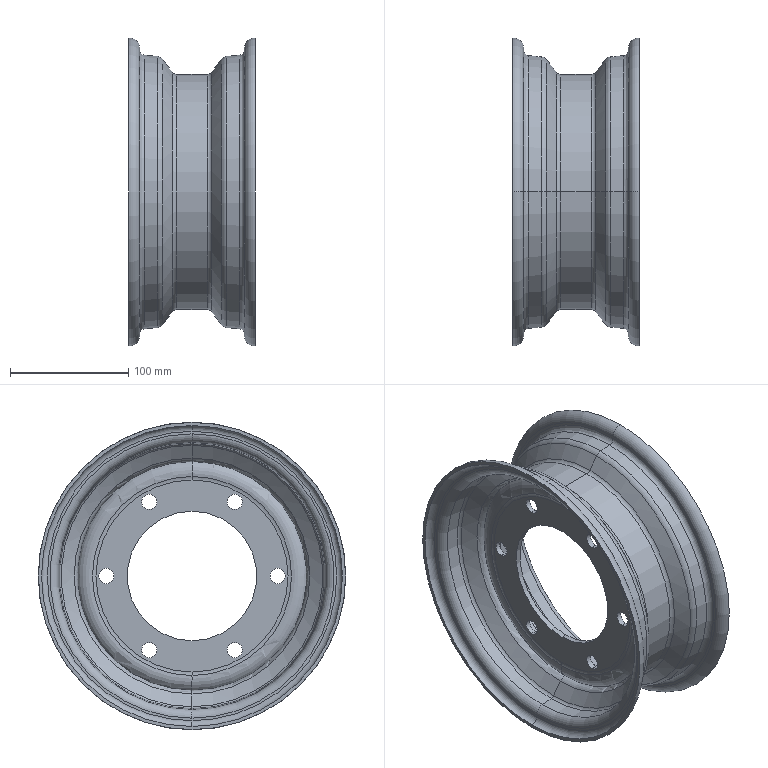Part | SolidWorks | features ICE 2, Revolution 1, Scale 1 | 1 solid | 83 faces | box 106.97 x 260.313 x 260.313 mm | volume 368325 mm3 | torus 38 | cylinder 20 | cone 16 | plane 9 | commonest cylinder face diameters 13 x12 109.701 x2 186.051 x2 193.826 x2 199.069 x2